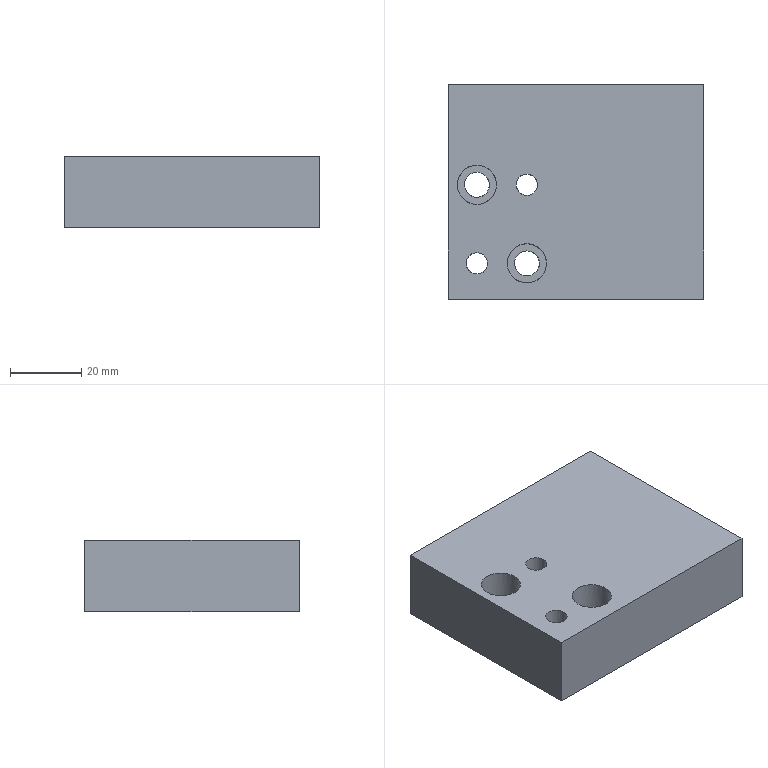Part | NX | features DIE-106 2 | 1 solid | 18 faces | box 71.5 x 60 x 20 mm | volume 81944 mm3 | plane 8 | cylinder 8 | cone 2 | commonest cylinder face diameters 3.506 x2 6 x2 7.007 x2 11 x2
STEP:
#1=CARTESIAN_POINT('',(4387.594,-904.372,894.343));
#2=VERTEX_POINT('',#1);
#3=CARTESIAN_POINT('',(4387.594,-844.372,894.343));
#4=VERTEX_POINT('',#3);
#5=CARTESIAN_POINT('',(4387.594,-863.648,894.343));
#6=DIRECTION('',(0.,1.,0.));
#7=VECTOR('',#6,1000.);
#8=LINE('',#5,#7);
#9=EDGE_CURVE('',#2,#4,#8,.T.);
#10=ORIENTED_EDGE('',*,*,#9,.F.);
#11=CARTESIAN_POINT('',(4387.594,-904.372,914.343));
#12=VERTEX_POINT('',#11);
#13=CARTESIAN_POINT('',(4387.594,-904.372,880.343));
#14=DIRECTION('',(0.,0.,1.));
#15=VECTOR('',#14,1000.);
#16=LINE('',#13,#15);
#17=EDGE_CURVE('',#2,#12,#16,.T.);
#18=ORIENTED_EDGE('',*,*,#17,.T.);
#19=CARTESIAN_POINT('',(4387.594,-844.372,914.343));
#20=VERTEX_POINT('',#19);
#21=CARTESIAN_POINT('',(4387.594,-895.398,914.343));
#22=DIRECTION('',(0.,1.,0.));
#23=VECTOR('',#22,1000.);
#24=LINE('',#21,#23);
#25=EDGE_CURVE('',#12,#20,#24,.T.);
#26=ORIENTED_EDGE('',*,*,#25,.T.);
#27=CARTESIAN_POINT('',(4387.594,-844.372,880.343));
#28=DIRECTION('',(0.,0.,-1.));
#29=VECTOR('',#28,1000.);
#30=LINE('',#27,#29);
#31=EDGE_CURVE('',#20,#4,#30,.T.);
#32=ORIENTED_EDGE('',*,*,#31,.T.);
#33=EDGE_LOOP('',(#10,#18,#26,#32));
#34=FACE_BOUND('',#33,.T.);
#35=CARTESIAN_POINT('',(4387.594,-863.648,880.343));
#36=DIRECTION('',(-1.,0.,0.));
#37=DIRECTION('',(0.,0.,-1.));
#38=AXIS2_PLACEMENT_3D('',#35,#36,#37);
#39=PLANE('',#38);
#40=ADVANCED_FACE('',(#34),#39,.T.);
#41=CARTESIAN_POINT('',(4459.094,-844.372,914.343));
#42=VERTEX_POINT('',#41);
#43=CARTESIAN_POINT('',(4374.094,-844.372,914.343));
#44=DIRECTION('',(1.,0.,0.));
#45=VECTOR('',#44,1000.);
#46=LINE('',#43,#45);
#47=EDGE_CURVE('',#20,#42,#46,.T.);
#48=ORIENTED_EDGE('',*,*,#47,.T.);
#49=CARTESIAN_POINT('',(4459.094,-844.372,894.343));
#50=VERTEX_POINT('',#49);
#51=CARTESIAN_POINT('',(4459.094,-844.372,880.343));
#52=DIRECTION('',(0.,0.,-1.));
#53=VECTOR('',#52,1000.);
#54=LINE('',#51,#53);
#55=EDGE_CURVE('',#42,#50,#54,.T.);
#56=ORIENTED_EDGE('',*,*,#55,.T.);
#57=CARTESIAN_POINT('',(4374.094,-844.372,894.343));
#58=DIRECTION('',(-1.,0.,0.));
#59=VECTOR('',#58,1000.);
#60=LINE('',#57,#59);
#61=EDGE_CURVE('',#50,#4,#60,.T.);
#62=ORIENTED_EDGE('',*,*,#61,.T.);
#63=ORIENTED_EDGE('',*,*,#31,.F.);
#64=EDGE_LOOP('',(#48,#56,#62,#63));
#65=FACE_BOUND('',#64,.T.);
#66=CARTESIAN_POINT('',(4374.094,-844.372,880.343));
#67=DIRECTION('',(0.,1.,0.));
#68=DIRECTION('',(0.,0.,-1.));
#69=AXIS2_PLACEMENT_3D('',#66,#67,#68);
#70=PLANE('',#69);
#71=ADVANCED_FACE('',(#65),#70,.T.);
#72=CARTESIAN_POINT('',(4459.094,-904.372,894.343));
#73=VERTEX_POINT('',#72);
#74=CARTESIAN_POINT('',(4446.464,-904.372,894.343));
#75=DIRECTION('',(1.,0.,0.));
#76=VECTOR('',#75,1000.);
#77=LINE('',#74,#76);
#78=EDGE_CURVE('',#2,#73,#77,.T.);
#79=ORIENTED_EDGE('',*,*,#78,.T.);
#80=CARTESIAN_POINT('',(4459.094,-904.372,914.343));
#81=VERTEX_POINT('',#80);
#82=CARTESIAN_POINT('',(4459.094,-904.372,880.343));
#83=DIRECTION('',(0.,0.,-1.));
#84=VECTOR('',#83,1000.);
#85=LINE('',#82,#84);
#86=EDGE_CURVE('',#81,#73,#85,.T.);
#87=ORIENTED_EDGE('',*,*,#86,.F.);
#88=CARTESIAN_POINT('',(4404.094,-904.372,914.343));
#89=DIRECTION('',(-1.,0.,0.));
#90=VECTOR('',#89,1000.);
#91=LINE('',#88,#90);
#92=EDGE_CURVE('',#81,#12,#91,.T.);
#93=ORIENTED_EDGE('',*,*,#92,.T.);
#94=ORIENTED_EDGE('',*,*,#17,.F.);
#95=EDGE_LOOP('',(#79,#87,#93,#94));
#96=FACE_BOUND('',#95,.T.);
#97=CARTESIAN_POINT('',(4374.094,-904.372,880.343));
#98=DIRECTION('',(0.,-1.,0.));
#99=DIRECTION('',(0.,0.,1.));
#100=AXIS2_PLACEMENT_3D('',#97,#98,#99);
#101=PLANE('',#100);
#102=ADVANCED_FACE('',(#96),#101,.T.);
#103=CARTESIAN_POINT('',(4409.594,-869.372,894.343));
#104=VERTEX_POINT('',#103);
#105=CARTESIAN_POINT('',(4409.594,-872.372,894.343));
#106=DIRECTION('',(0.,0.,1.));
#107=DIRECTION('',(0.,1.,0.));
#108=AXIS2_PLACEMENT_3D('',#105,#106,#107);
#109=CIRCLE('',#108,3.);
#110=EDGE_CURVE('',#104,#104,#109,.T.);
#111=ORIENTED_EDGE('',*,*,#110,.T.);
#112=EDGE_LOOP('',(#111));
#113=FACE_BOUND('',#112,.T.);
#114=CARTESIAN_POINT('',(4395.594,-891.372,894.343));
#115=VERTEX_POINT('',#114);
#116=CARTESIAN_POINT('',(4395.594,-894.372,894.343));
#117=DIRECTION('',(0.,0.,1.));
#118=DIRECTION('',(0.,1.,0.));
#119=AXIS2_PLACEMENT_3D('',#116,#117,#118);
#120=CIRCLE('',#119,3.);
#121=EDGE_CURVE('',#115,#115,#120,.T.);
#122=ORIENTED_EDGE('',*,*,#121,.T.);
#123=EDGE_LOOP('',(#122));
#124=FACE_BOUND('',#123,.T.);
#125=CARTESIAN_POINT('',(4395.594,-868.869,894.343));
#126=VERTEX_POINT('',#125);
#127=CARTESIAN_POINT('',(4395.594,-872.372,894.343));
#128=DIRECTION('',(0.,0.,1.));
#129=DIRECTION('',(0.,1.,0.));
#130=AXIS2_PLACEMENT_3D('',#127,#128,#129);
#131=CIRCLE('',#130,3.503);
#132=EDGE_CURVE('',#126,#126,#131,.T.);
#133=ORIENTED_EDGE('',*,*,#132,.T.);
#134=EDGE_LOOP('',(#133));
#135=FACE_BOUND('',#134,.T.);
#136=CARTESIAN_POINT('',(4409.594,-890.869,894.343));
#137=VERTEX_POINT('',#136);
#138=CARTESIAN_POINT('',(4409.594,-894.372,894.343));
#139=DIRECTION('',(0.,0.,1.));
#140=DIRECTION('',(0.,1.,0.));
#141=AXIS2_PLACEMENT_3D('',#138,#139,#140);
#142=CIRCLE('',#141,3.503);
#143=EDGE_CURVE('',#137,#137,#142,.T.);
#144=ORIENTED_EDGE('',*,*,#143,.T.);
#145=EDGE_LOOP('',(#144));
#146=FACE_BOUND('',#145,.T.);
#147=ORIENTED_EDGE('',*,*,#61,.F.);
#148=CARTESIAN_POINT('',(4459.094,-1000.372,894.343));
#149=DIRECTION('',(0.,1.,0.));
#150=VECTOR('',#149,1000.);
#151=LINE('',#148,#150);
#152=EDGE_CURVE('',#73,#50,#151,.T.);
#153=ORIENTED_EDGE('',*,*,#152,.F.);
#154=ORIENTED_EDGE('',*,*,#78,.F.);
#155=ORIENTED_EDGE('',*,*,#9,.T.);
#156=EDGE_LOOP('',(#147,#153,#154,#155));
#157=FACE_BOUND('',#156,.T.);
#158=CARTESIAN_POINT('',(4449.945,-856.298,894.343));
#159=VERTEX_POINT('',#158);
#160=CARTESIAN_POINT('',(4448.192,-856.298,894.343));
#161=DIRECTION('',(0.,0.,1.));
#162=DIRECTION('',(1.,0.,0.));
#163=AXIS2_PLACEMENT_3D('',#160,#161,#162);
#164=CIRCLE('',#163,1.753);
#165=EDGE_CURVE('',#159,#159,#164,.T.);
#166=ORIENTED_EDGE('',*,*,#165,.T.);
#167=EDGE_LOOP('',(#166));
#168=FACE_BOUND('',#167,.T.);
#169=CARTESIAN_POINT('',(4449.945,-881.698,894.343));
#170=VERTEX_POINT('',#169);
#171=CARTESIAN_POINT('',(4448.192,-881.698,894.343));
#172=DIRECTION('',(0.,0.,1.));
#173=DIRECTION('',(1.,0.,0.));
#174=AXIS2_PLACEMENT_3D('',#171,#172,#173);
#175=CIRCLE('',#174,1.753);
#176=EDGE_CURVE('',#170,#170,#175,.T.);
#177=ORIENTED_EDGE('',*,*,#176,.T.);
#178=EDGE_LOOP('',(#177));
#179=FACE_BOUND('',#178,.T.);
#180=CARTESIAN_POINT('',(4446.464,-884.398,894.343));
#181=DIRECTION('',(0.,0.,1.));
#182=DIRECTION('',(-1.,0.,0.));
#183=AXIS2_PLACEMENT_3D('',#180,#181,#182);
#184=PLANE('',#183);
#185=ADVANCED_FACE('',(#113,#124,#135,#146,#157,#168,#179),#184,.F.);
#186=CARTESIAN_POINT('',(4406.594,-872.372,914.343));
#187=VERTEX_POINT('',#186);
#188=CARTESIAN_POINT('',(4409.594,-872.372,914.343));
#189=DIRECTION('',(0.,0.,-1.));
#190=DIRECTION('',(-1.,0.,0.));
#191=AXIS2_PLACEMENT_3D('',#188,#189,#190);
#192=CIRCLE('',#191,3.);
#193=EDGE_CURVE('',#187,#187,#192,.T.);
#194=ORIENTED_EDGE('',*,*,#193,.T.);
#195=EDGE_LOOP('',(#194));
#196=FACE_BOUND('',#195,.T.);
#197=CARTESIAN_POINT('',(4392.594,-894.372,914.343));
#198=VERTEX_POINT('',#197);
#199=CARTESIAN_POINT('',(4395.594,-894.372,914.343));
#200=DIRECTION('',(0.,0.,-1.));
#201=DIRECTION('',(-1.,0.,0.));
#202=AXIS2_PLACEMENT_3D('',#199,#200,#201);
#203=CIRCLE('',#202,3.);
#204=EDGE_CURVE('',#198,#198,#203,.T.);
#205=ORIENTED_EDGE('',*,*,#204,.T.);
#206=EDGE_LOOP('',(#205));
#207=FACE_BOUND('',#206,.T.);
#208=CARTESIAN_POINT('',(4390.094,-872.372,914.343));
#209=VERTEX_POINT('',#208);
#210=CARTESIAN_POINT('',(4395.594,-872.372,914.343));
#211=DIRECTION('',(0.,0.,-1.));
#212=DIRECTION('',(-1.,0.,0.));
#213=AXIS2_PLACEMENT_3D('',#210,#211,#212);
#214=CIRCLE('',#213,5.5);
#215=EDGE_CURVE('',#209,#209,#214,.T.);
#216=ORIENTED_EDGE('',*,*,#215,.T.);
#217=EDGE_LOOP('',(#216));
#218=FACE_BOUND('',#217,.T.);
#219=CARTESIAN_POINT('',(4404.094,-894.372,914.343));
#220=VERTEX_POINT('',#219);
#221=CARTESIAN_POINT('',(4409.594,-894.372,914.343));
#222=DIRECTION('',(0.,0.,-1.));
#223=DIRECTION('',(-1.,0.,0.));
#224=AXIS2_PLACEMENT_3D('',#221,#222,#223);
#225=CIRCLE('',#224,5.5);
#226=EDGE_CURVE('',#220,#220,#225,.T.);
#227=ORIENTED_EDGE('',*,*,#226,.T.);
#228=EDGE_LOOP('',(#227));
#229=FACE_BOUND('',#228,.T.);
#230=ORIENTED_EDGE('',*,*,#92,.F.);
#231=CARTESIAN_POINT('',(4459.094,-1000.372,914.343));
#232=DIRECTION('',(0.,-1.,0.));
#233=VECTOR('',#232,1000.);
#234=LINE('',#231,#233);
#235=EDGE_CURVE('',#42,#81,#234,.T.);
#236=ORIENTED_EDGE('',*,*,#235,.F.);
#237=ORIENTED_EDGE('',*,*,#47,.F.);
#238=ORIENTED_EDGE('',*,*,#25,.F.);
#239=EDGE_LOOP('',(#230,#236,#237,#238));
#240=FACE_BOUND('',#239,.T.);
#241=CARTESIAN_POINT('',(4404.094,-895.398,914.343));
#242=DIRECTION('',(0.,0.,-1.));
#243=DIRECTION('',(0.,-1.,0.));
#244=AXIS2_PLACEMENT_3D('',#241,#242,#243);
#245=PLANE('',#244);
#246=ADVANCED_FACE('',(#196,#207,#218,#229,#240),#245,.F.);
#247=CARTESIAN_POINT('',(4409.594,-888.872,905.343));
#248=VERTEX_POINT('',#247);
#249=CARTESIAN_POINT('',(4409.594,-894.372,905.343));
#250=DIRECTION('',(0.,0.,-1.));
#251=DIRECTION('',(0.,1.,0.));
#252=AXIS2_PLACEMENT_3D('',#249,#250,#251);
#253=CIRCLE('',#252,5.5);
#254=EDGE_CURVE('',#248,#248,#253,.T.);
#255=ORIENTED_EDGE('',*,*,#254,.T.);
#256=EDGE_LOOP('',(#255));
#257=FACE_BOUND('',#256,.T.);
#258=ORIENTED_EDGE('',*,*,#226,.F.);
#259=EDGE_LOOP('',(#258));
#260=FACE_BOUND('',#259,.T.);
#261=CARTESIAN_POINT('',(4409.594,-894.372,905.343));
#262=DIRECTION('',(0.,0.,1.));
#263=DIRECTION('',(-1.,0.,0.));
#264=AXIS2_PLACEMENT_3D('',#261,#262,#263);
#265=CYLINDRICAL_SURFACE('',#264,5.5);
#266=ADVANCED_FACE('',(#257,#260),#265,.F.);
#267=ORIENTED_EDGE('',*,*,#143,.F.);
#268=EDGE_LOOP('',(#267));
#269=FACE_BOUND('',#268,.T.);
#270=CARTESIAN_POINT('',(4413.097,-894.372,905.343));
#271=VERTEX_POINT('',#270);
#272=CARTESIAN_POINT('',(4409.594,-894.372,905.343));
#273=DIRECTION('',(0.,0.,1.));
#274=DIRECTION('',(1.,0.,0.));
#275=AXIS2_PLACEMENT_3D('',#272,#273,#274);
#276=CIRCLE('',#275,3.503);
#277=EDGE_CURVE('',#271,#271,#276,.T.);
#278=ORIENTED_EDGE('',*,*,#277,.T.);
#279=EDGE_LOOP('',(#278));
#280=FACE_BOUND('',#279,.T.);
#281=CARTESIAN_POINT('',(4409.594,-894.372,894.343));
#282=DIRECTION('',(0.,0.,1.));
#283=DIRECTION('',(-1.,0.,0.));
#284=AXIS2_PLACEMENT_3D('',#281,#282,#283);
#285=CYLINDRICAL_SURFACE('',#284,3.503);
#286=ADVANCED_FACE('',(#269,#280),#285,.F.);
#287=ORIENTED_EDGE('',*,*,#277,.F.);
#288=EDGE_LOOP('',(#287));
#289=FACE_BOUND('',#288,.T.);
#290=ORIENTED_EDGE('',*,*,#254,.F.);
#291=EDGE_LOOP('',(#290));
#292=FACE_BOUND('',#291,.T.);
#293=CARTESIAN_POINT('',(4409.594,-894.372,905.343));
#294=DIRECTION('',(0.,0.,1.));
#295=DIRECTION('',(-1.,0.,0.));
#296=AXIS2_PLACEMENT_3D('',#293,#294,#295);
#297=PLANE('',#296);
#298=ADVANCED_FACE('',(#289,#292),#297,.T.);
#299=CARTESIAN_POINT('',(4395.594,-866.872,905.343));
#300=VERTEX_POINT('',#299);
#301=CARTESIAN_POINT('',(4395.594,-872.372,905.343));
#302=DIRECTION('',(0.,0.,-1.));
#303=DIRECTION('',(0.,1.,0.));
#304=AXIS2_PLACEMENT_3D('',#301,#302,#303);
#305=CIRCLE('',#304,5.5);
#306=EDGE_CURVE('',#300,#300,#305,.T.);
#307=ORIENTED_EDGE('',*,*,#306,.T.);
#308=EDGE_LOOP('',(#307));
#309=FACE_BOUND('',#308,.T.);
#310=ORIENTED_EDGE('',*,*,#215,.F.);
#311=EDGE_LOOP('',(#310));
#312=FACE_BOUND('',#311,.T.);
#313=CARTESIAN_POINT('',(4395.594,-872.372,905.343));
#314=DIRECTION('',(0.,0.,1.));
#315=DIRECTION('',(-1.,0.,0.));
#316=AXIS2_PLACEMENT_3D('',#313,#314,#315);
#317=CYLINDRICAL_SURFACE('',#316,5.5);
#318=ADVANCED_FACE('',(#309,#312),#317,.F.);
#319=ORIENTED_EDGE('',*,*,#132,.F.);
#320=EDGE_LOOP('',(#319));
#321=FACE_BOUND('',#320,.T.);
#322=CARTESIAN_POINT('',(4399.097,-872.372,905.343));
#323=VERTEX_POINT('',#322);
#324=CARTESIAN_POINT('',(4395.594,-872.372,905.343));
#325=DIRECTION('',(0.,0.,1.));
#326=DIRECTION('',(1.,0.,0.));
#327=AXIS2_PLACEMENT_3D('',#324,#325,#326);
#328=CIRCLE('',#327,3.503);
#329=EDGE_CURVE('',#323,#323,#328,.T.);
#330=ORIENTED_EDGE('',*,*,#329,.T.);
#331=EDGE_LOOP('',(#330));
#332=FACE_BOUND('',#331,.T.);
#333=CARTESIAN_POINT('',(4395.594,-872.372,894.343));
#334=DIRECTION('',(0.,0.,1.));
#335=DIRECTION('',(-1.,0.,0.));
#336=AXIS2_PLACEMENT_3D('',#333,#334,#335);
#337=CYLINDRICAL_SURFACE('',#336,3.503);
#338=ADVANCED_FACE('',(#321,#332),#337,.F.);
#339=ORIENTED_EDGE('',*,*,#329,.F.);
#340=EDGE_LOOP('',(#339));
#341=FACE_BOUND('',#340,.T.);
#342=ORIENTED_EDGE('',*,*,#306,.F.);
#343=EDGE_LOOP('',(#342));
#344=FACE_BOUND('',#343,.T.);
#345=CARTESIAN_POINT('',(4395.594,-872.372,905.343));
#346=DIRECTION('',(0.,0.,1.));
#347=DIRECTION('',(-1.,0.,0.));
#348=AXIS2_PLACEMENT_3D('',#345,#346,#347);
#349=PLANE('',#348);
#350=ADVANCED_FACE('',(#341,#344),#349,.T.);
#351=ORIENTED_EDGE('',*,*,#121,.F.);
#352=EDGE_LOOP('',(#351));
#353=FACE_BOUND('',#352,.T.);
#354=ORIENTED_EDGE('',*,*,#204,.F.);
#355=EDGE_LOOP('',(#354));
#356=FACE_BOUND('',#355,.T.);
#357=CARTESIAN_POINT('',(4395.594,-894.372,894.343));
#358=DIRECTION('',(0.,0.,1.));
#359=DIRECTION('',(-1.,0.,0.));
#360=AXIS2_PLACEMENT_3D('',#357,#358,#359);
#361=CYLINDRICAL_SURFACE('',#360,3.);
#362=ADVANCED_FACE('',(#353,#356),#361,.F.);
#363=ORIENTED_EDGE('',*,*,#110,.F.);
#364=EDGE_LOOP('',(#363));
#365=FACE_BOUND('',#364,.T.);
#366=ORIENTED_EDGE('',*,*,#193,.F.);
#367=EDGE_LOOP('',(#366));
#368=FACE_BOUND('',#367,.T.);
#369=CARTESIAN_POINT('',(4409.594,-872.372,894.343));
#370=DIRECTION('',(0.,0.,1.));
#371=DIRECTION('',(-1.,0.,0.));
#372=AXIS2_PLACEMENT_3D('',#369,#370,#371);
#373=CYLINDRICAL_SURFACE('',#372,3.);
#374=ADVANCED_FACE('',(#365,#368),#373,.F.);
#375=ORIENTED_EDGE('',*,*,#86,.T.);
#376=ORIENTED_EDGE('',*,*,#152,.T.);
#377=ORIENTED_EDGE('',*,*,#55,.F.);
#378=ORIENTED_EDGE('',*,*,#235,.T.);
#379=EDGE_LOOP('',(#375,#376,#377,#378));
#380=FACE_BOUND('',#379,.T.);
#381=CARTESIAN_POINT('',(4459.094,-1000.372,815.716));
#382=DIRECTION('',(-1.,0.,0.));
#383=DIRECTION('',(0.,-1.,0.));
#384=AXIS2_PLACEMENT_3D('',#381,#382,#383);
#385=PLANE('',#384);
#386=ADVANCED_FACE('',(#380),#385,.F.);
#387=CARTESIAN_POINT('',(4449.945,-881.698,902.343));
#388=VERTEX_POINT('',#387);
#389=CARTESIAN_POINT('',(4448.192,-881.698,902.343));
#390=DIRECTION('',(0.,0.,1.));
#391=DIRECTION('',(1.,0.,0.));
#392=AXIS2_PLACEMENT_3D('',#389,#390,#391);
#393=CIRCLE('',#392,1.753);
#394=EDGE_CURVE('',#388,#388,#393,.T.);
#395=ORIENTED_EDGE('',*,*,#394,.T.);
#396=EDGE_LOOP('',(#395));
#397=FACE_BOUND('',#396,.T.);
#398=ORIENTED_EDGE('',*,*,#176,.F.);
#399=EDGE_LOOP('',(#398));
#400=FACE_BOUND('',#399,.T.);
#401=CARTESIAN_POINT('',(4448.192,-881.698,894.343));
#402=DIRECTION('',(0.,0.,1.));
#403=DIRECTION('',(-1.,0.,0.));
#404=AXIS2_PLACEMENT_3D('',#401,#402,#403);
#405=CYLINDRICAL_SURFACE('',#404,1.753);
#406=ADVANCED_FACE('',(#397,#400),#405,.F.);
#407=CARTESIAN_POINT('',(4448.192,-881.698,904.096));
#408=VERTEX_POINT('',#407);
#409=VERTEX_LOOP('',#408);
#410=FACE_BOUND('',#409,.T.);
#411=ORIENTED_EDGE('',*,*,#394,.F.);
#412=EDGE_LOOP('',(#411));
#413=FACE_BOUND('',#412,.T.);
#414=CARTESIAN_POINT('',(4448.192,-881.698,902.343));
#415=DIRECTION('',(0.,0.,-1.));
#416=DIRECTION('',(1.,0.,0.));
#417=AXIS2_PLACEMENT_3D('',#414,#415,#416);
#418=CONICAL_SURFACE('',#417,1.753,0.7854);
#419=ADVANCED_FACE('',(#410,#413),#418,.F.);
#420=CARTESIAN_POINT('',(4449.945,-856.298,902.343));
#421=VERTEX_POINT('',#420);
#422=CARTESIAN_POINT('',(4448.192,-856.298,902.343));
#423=DIRECTION('',(0.,0.,1.));
#424=DIRECTION('',(1.,0.,0.));
#425=AXIS2_PLACEMENT_3D('',#422,#423,#424);
#426=CIRCLE('',#425,1.753);
#427=EDGE_CURVE('',#421,#421,#426,.T.);
#428=ORIENTED_EDGE('',*,*,#427,.T.);
#429=EDGE_LOOP('',(#428));
#430=FACE_BOUND('',#429,.T.);
#431=ORIENTED_EDGE('',*,*,#165,.F.);
#432=EDGE_LOOP('',(#431));
#433=FACE_BOUND('',#432,.T.);
#434=CARTESIAN_POINT('',(4448.192,-856.298,894.343));
#435=DIRECTION('',(0.,0.,1.));
#436=DIRECTION('',(-1.,0.,0.));
#437=AXIS2_PLACEMENT_3D('',#434,#435,#436);
#438=CYLINDRICAL_SURFACE('',#437,1.753);
#439=ADVANCED_FACE('',(#430,#433),#438,.F.);
#440=CARTESIAN_POINT('',(4448.192,-856.298,904.096));
#441=VERTEX_POINT('',#440);
#442=VERTEX_LOOP('',#441);
#443=FACE_BOUND('',#442,.T.);
#444=ORIENTED_EDGE('',*,*,#427,.F.);
#445=EDGE_LOOP('',(#444));
#446=FACE_BOUND('',#445,.T.);
#447=CARTESIAN_POINT('',(4448.192,-856.298,902.343));
#448=DIRECTION('',(0.,0.,-1.));
#449=DIRECTION('',(1.,0.,0.));
#450=AXIS2_PLACEMENT_3D('',#447,#448,#449);
#451=CONICAL_SURFACE('',#450,1.753,0.7854);
#452=ADVANCED_FACE('',(#443,#446),#451,.F.);
#453=CLOSED_SHELL('',(#40,#71,#102,#185,#246,#266,#286,#298,#318,#338,#350,#362,#374,#386,#406,#419,#439,#452));
#454=MANIFOLD_SOLID_BREP('',#453);
#455=(LENGTH_UNIT()NAMED_UNIT(*)SI_UNIT(.MILLI.,.METRE.));
#456=UNCERTAINTY_MEASURE_WITH_UNIT(LENGTH_MEASURE(0.00001),#455,'','');
#457=(NAMED_UNIT(*)PLANE_ANGLE_UNIT()SI_UNIT($,.RADIAN.));
#458=(NAMED_UNIT(*)SI_UNIT($,.STERADIAN.)SOLID_ANGLE_UNIT());
#459=(GEOMETRIC_REPRESENTATION_CONTEXT(3)GLOBAL_UNCERTAINTY_ASSIGNED_CONTEXT((#456))GLOBAL_UNIT_ASSIGNED_CONTEXT((#455,#457,#458))REPRESENTATION_CONTEXT('',''));
#460=ADVANCED_BREP_SHAPE_REPRESENTATION('',(#454),#459);